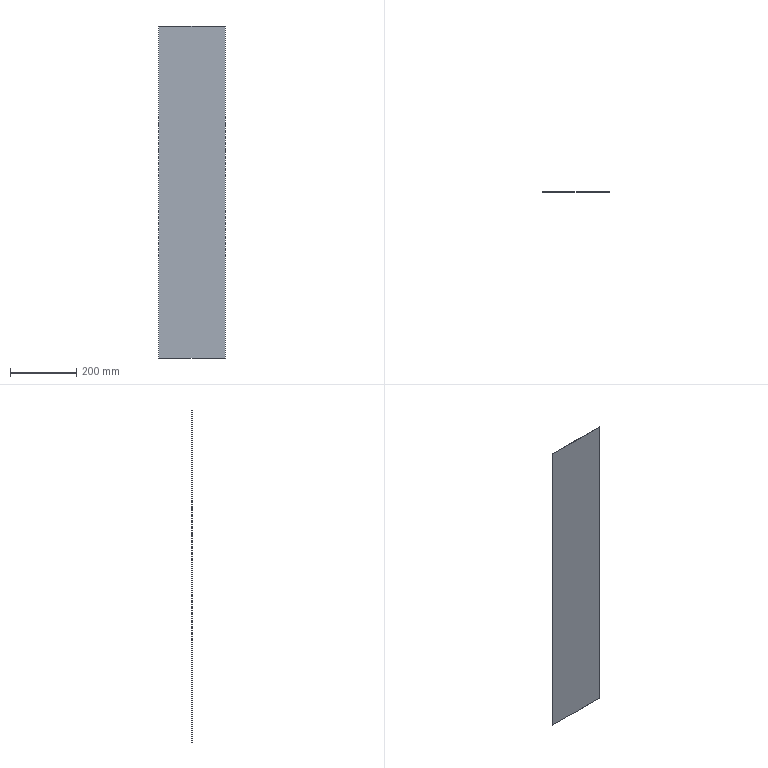Part | SolidWorks | features Extrusion 1 | 1 solid | 6 faces | box 200 x 1 x 1000 mm | volume 200000 mm3 | plane 6
STEP:
#1=CARTESIAN_POINT('',(100.,0.,500.));
#2=VERTEX_POINT('',#1);
#3=CARTESIAN_POINT('',(100.,0.,-500.));
#4=VERTEX_POINT('',#3);
#5=CARTESIAN_POINT('',(100.,0.,500.));
#6=DIRECTION('',(0.,0.,-1.));
#7=VECTOR('',#6,1000.);
#8=LINE('',#5,#7);
#9=EDGE_CURVE('',#2,#4,#8,.T.);
#10=ORIENTED_EDGE('',*,*,#9,.T.);
#11=CARTESIAN_POINT('',(100.,1.,-500.));
#12=VERTEX_POINT('',#11);
#13=CARTESIAN_POINT('',(100.,1.,-500.));
#14=DIRECTION('',(0.,-1.,0.));
#15=VECTOR('',#14,1000.);
#16=LINE('',#13,#15);
#17=EDGE_CURVE('',#12,#4,#16,.T.);
#18=ORIENTED_EDGE('',*,*,#17,.F.);
#19=CARTESIAN_POINT('',(100.,1.,500.));
#20=VERTEX_POINT('',#19);
#21=CARTESIAN_POINT('',(100.,1.,500.));
#22=DIRECTION('',(0.,0.,-1.));
#23=VECTOR('',#22,1000.);
#24=LINE('',#21,#23);
#25=EDGE_CURVE('',#20,#12,#24,.T.);
#26=ORIENTED_EDGE('',*,*,#25,.F.);
#27=CARTESIAN_POINT('',(100.,1.,500.));
#28=DIRECTION('',(0.,-1.,0.));
#29=VECTOR('',#28,1000.);
#30=LINE('',#27,#29);
#31=EDGE_CURVE('',#20,#2,#30,.T.);
#32=ORIENTED_EDGE('',*,*,#31,.T.);
#33=EDGE_LOOP('',(#10,#18,#26,#32));
#34=FACE_OUTER_BOUND('',#33,.T.);
#35=CARTESIAN_POINT('',(100.,1.,500.));
#36=DIRECTION('',(-1.,0.,0.));
#37=DIRECTION('',(0.,0.,1.));
#38=AXIS2_PLACEMENT_3D('',#35,#36,#37);
#39=PLANE('',#38);
#40=ADVANCED_FACE('',(#34),#39,.F.);
#41=CARTESIAN_POINT('',(-100.,0.,-500.));
#42=VERTEX_POINT('',#41);
#43=CARTESIAN_POINT('',(-100.,0.,-500.));
#44=DIRECTION('',(-1.,0.,0.));
#45=VECTOR('',#44,1000.);
#46=LINE('',#43,#45);
#47=EDGE_CURVE('',#4,#42,#46,.T.);
#48=ORIENTED_EDGE('',*,*,#47,.T.);
#49=CARTESIAN_POINT('',(-100.,1.,-500.));
#50=VERTEX_POINT('',#49);
#51=CARTESIAN_POINT('',(-100.,1.,-500.));
#52=DIRECTION('',(0.,-1.,0.));
#53=VECTOR('',#52,1000.);
#54=LINE('',#51,#53);
#55=EDGE_CURVE('',#50,#42,#54,.T.);
#56=ORIENTED_EDGE('',*,*,#55,.F.);
#57=CARTESIAN_POINT('',(-100.,1.,-500.));
#58=DIRECTION('',(-1.,0.,0.));
#59=VECTOR('',#58,1000.);
#60=LINE('',#57,#59);
#61=EDGE_CURVE('',#12,#50,#60,.T.);
#62=ORIENTED_EDGE('',*,*,#61,.F.);
#63=ORIENTED_EDGE('',*,*,#17,.T.);
#64=EDGE_LOOP('',(#48,#56,#62,#63));
#65=FACE_OUTER_BOUND('',#64,.T.);
#66=CARTESIAN_POINT('',(-100.,1.,-500.));
#67=DIRECTION('',(0.,0.,1.));
#68=DIRECTION('',(1.,0.,0.));
#69=AXIS2_PLACEMENT_3D('',#66,#67,#68);
#70=PLANE('',#69);
#71=ADVANCED_FACE('',(#65),#70,.F.);
#72=CARTESIAN_POINT('',(-100.,0.,500.));
#73=VERTEX_POINT('',#72);
#74=CARTESIAN_POINT('',(-100.,0.,500.));
#75=DIRECTION('',(0.,0.,1.));
#76=VECTOR('',#75,1000.);
#77=LINE('',#74,#76);
#78=EDGE_CURVE('',#42,#73,#77,.T.);
#79=ORIENTED_EDGE('',*,*,#78,.T.);
#80=CARTESIAN_POINT('',(-100.,1.,500.));
#81=VERTEX_POINT('',#80);
#82=CARTESIAN_POINT('',(-100.,1.,500.));
#83=DIRECTION('',(0.,-1.,0.));
#84=VECTOR('',#83,1000.);
#85=LINE('',#82,#84);
#86=EDGE_CURVE('',#81,#73,#85,.T.);
#87=ORIENTED_EDGE('',*,*,#86,.F.);
#88=CARTESIAN_POINT('',(-100.,1.,500.));
#89=DIRECTION('',(0.,0.,1.));
#90=VECTOR('',#89,1000.);
#91=LINE('',#88,#90);
#92=EDGE_CURVE('',#50,#81,#91,.T.);
#93=ORIENTED_EDGE('',*,*,#92,.F.);
#94=ORIENTED_EDGE('',*,*,#55,.T.);
#95=EDGE_LOOP('',(#79,#87,#93,#94));
#96=FACE_OUTER_BOUND('',#95,.T.);
#97=CARTESIAN_POINT('',(-100.,1.,500.));
#98=DIRECTION('',(1.,0.,0.));
#99=DIRECTION('',(0.,0.,-1.));
#100=AXIS2_PLACEMENT_3D('',#97,#98,#99);
#101=PLANE('',#100);
#102=ADVANCED_FACE('',(#96),#101,.F.);
#103=CARTESIAN_POINT('',(-100.,0.,500.));
#104=DIRECTION('',(1.,0.,0.));
#105=VECTOR('',#104,1000.);
#106=LINE('',#103,#105);
#107=EDGE_CURVE('',#73,#2,#106,.T.);
#108=ORIENTED_EDGE('',*,*,#107,.T.);
#109=ORIENTED_EDGE('',*,*,#31,.F.);
#110=CARTESIAN_POINT('',(-100.,1.,500.));
#111=DIRECTION('',(1.,0.,0.));
#112=VECTOR('',#111,1000.);
#113=LINE('',#110,#112);
#114=EDGE_CURVE('',#81,#20,#113,.T.);
#115=ORIENTED_EDGE('',*,*,#114,.F.);
#116=ORIENTED_EDGE('',*,*,#86,.T.);
#117=EDGE_LOOP('',(#108,#109,#115,#116));
#118=FACE_OUTER_BOUND('',#117,.T.);
#119=CARTESIAN_POINT('',(-100.,1.,500.));
#120=DIRECTION('',(0.,0.,-1.));
#121=DIRECTION('',(-1.,0.,0.));
#122=AXIS2_PLACEMENT_3D('',#119,#120,#121);
#123=PLANE('',#122);
#124=ADVANCED_FACE('',(#118),#123,.F.);
#125=ORIENTED_EDGE('',*,*,#25,.T.);
#126=ORIENTED_EDGE('',*,*,#61,.T.);
#127=ORIENTED_EDGE('',*,*,#92,.T.);
#128=ORIENTED_EDGE('',*,*,#114,.T.);
#129=EDGE_LOOP('',(#125,#126,#127,#128));
#130=FACE_OUTER_BOUND('',#129,.T.);
#131=CARTESIAN_POINT('',(0.,1.,0.));
#132=DIRECTION('',(0.,-1.,0.));
#133=DIRECTION('',(0.,0.,-1.));
#134=AXIS2_PLACEMENT_3D('',#131,#132,#133);
#135=PLANE('',#134);
#136=ADVANCED_FACE('',(#130),#135,.F.);
#137=ORIENTED_EDGE('',*,*,#9,.F.);
#138=ORIENTED_EDGE('',*,*,#107,.F.);
#139=ORIENTED_EDGE('',*,*,#78,.F.);
#140=ORIENTED_EDGE('',*,*,#47,.F.);
#141=EDGE_LOOP('',(#137,#138,#139,#140));
#142=FACE_OUTER_BOUND('',#141,.T.);
#143=CARTESIAN_POINT('',(0.,0.,0.));
#144=DIRECTION('',(0.,-1.,0.));
#145=DIRECTION('',(0.,0.,-1.));
#146=AXIS2_PLACEMENT_3D('',#143,#144,#145);
#147=PLANE('',#146);
#148=ADVANCED_FACE('',(#142),#147,.T.);
#149=CLOSED_SHELL('',(#40,#71,#102,#124,#136,#148));
#150=MANIFOLD_SOLID_BREP('',#149);
#151=CARTESIAN_POINT('',(0.,0.,0.));
#152=DIRECTION('',(0.,0.,1.));
#153=DIRECTION('',(1.,0.,0.));
#154=AXIS2_PLACEMENT_3D('',#151,#152,#153);
#155=(LENGTH_UNIT()NAMED_UNIT(*)SI_UNIT(.MILLI.,.METRE.));
#156=UNCERTAINTY_MEASURE_WITH_UNIT(LENGTH_MEASURE(0.00001),#155,'','');
#157=(NAMED_UNIT(*)PLANE_ANGLE_UNIT()SI_UNIT($,.RADIAN.));
#158=(NAMED_UNIT(*)SI_UNIT($,.STERADIAN.)SOLID_ANGLE_UNIT());
#159=(GEOMETRIC_REPRESENTATION_CONTEXT(3)GLOBAL_UNCERTAINTY_ASSIGNED_CONTEXT((#156))GLOBAL_UNIT_ASSIGNED_CONTEXT((#155,#157,#158))REPRESENTATION_CONTEXT('',''));
#160=ADVANCED_BREP_SHAPE_REPRESENTATION('',(#150,#154),#159);